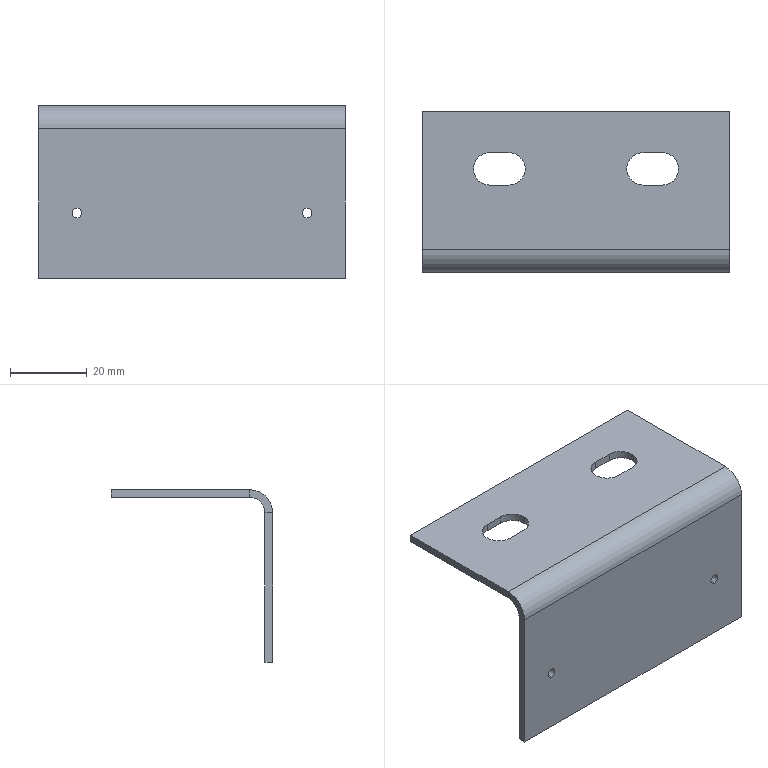Part | STEP file | PN_0019_default | 1 solid | 26 faces | box 80 x 42 x 45 mm | volume 12840 mm3 | plane 16 | cylinder 10 | commonest cylinder face diameters 2.5 x4 8.5 x4 8 x1 12 x1